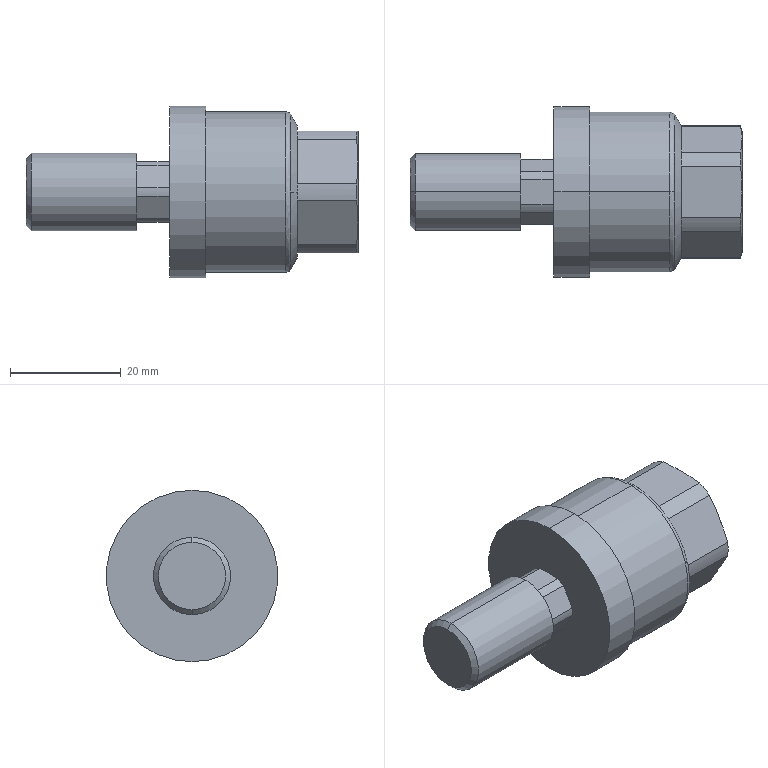Part | STEP file | 1 solid | 66 faces | box 60 x 31 x 31 mm | volume 22129 mm3 | plane 23 | cone 21 | cylinder 20 | spline 2 | commonest cylinder face diameters 11.9 x6 23.9 x6 12.376 x2 14 x2 29 x2 31 x2